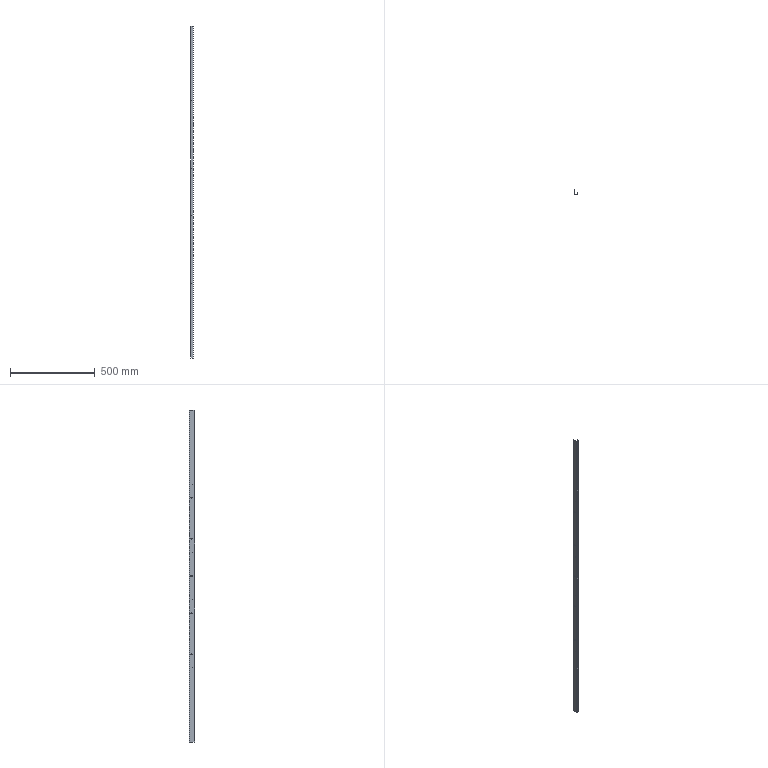Part | 1 solid | 72 faces | box 17 x 30 x 1956 mm | volume 153739 mm3 | plane 50 | cylinder 22 | commonest cylinder face diameters 6.1 x10 2 x6 5 x6